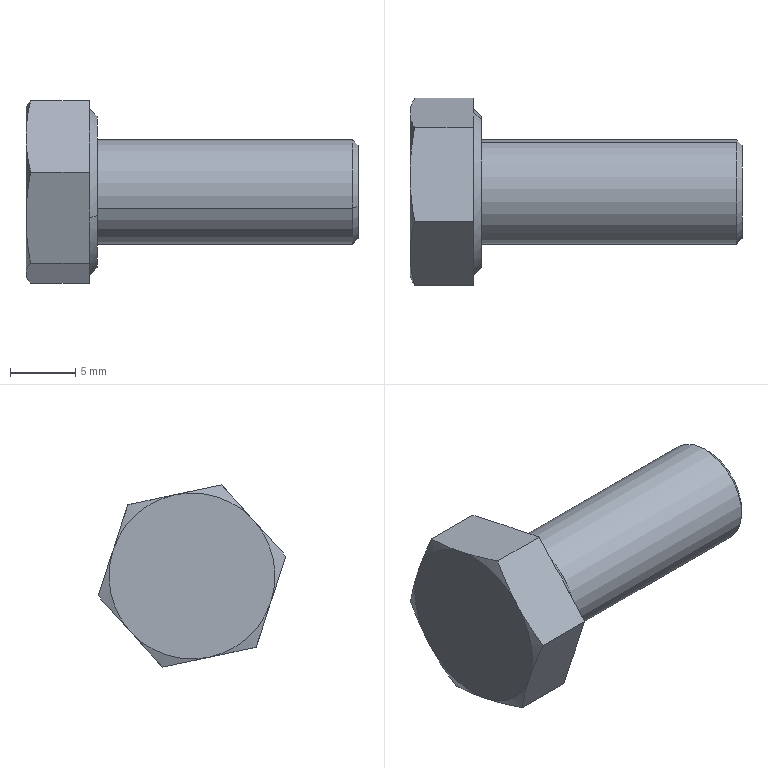Part | NX | features BREP 1 | 1 solid | 27 faces | box 25.45 x 14.378 x 13.98 mm | volume 1753 mm3 | plane 15 | cone 10 | cylinder 2 | commonest cylinder face diameters 8 x2
STEP:
#1=CARTESIAN_POINT('',(16.7,-2.901,82.764));
#2=VERTEX_POINT('',#1);
#3=CARTESIAN_POINT('',(16.7,3.946,84.989));
#4=VERTEX_POINT('',#3);
#5=CARTESIAN_POINT('',(16.7,0.5226,83.877));
#6=DIRECTION('',(1.,0.,0.));
#7=DIRECTION('',(0.,-0.9511,-0.309));
#8=AXIS2_PLACEMENT_3D('',#5,#6,#7);
#9=CIRCLE('',#8,3.6);
#10=EDGE_CURVE('',#2,#4,#9,.T.);
#11=ORIENTED_EDGE('',*,*,#10,.F.);
#12=CARTESIAN_POINT('',(16.3,-3.282,82.641));
#13=VERTEX_POINT('',#12);
#14=CARTESIAN_POINT('',(16.7,-2.901,82.764));
#15=DIRECTION('',(-0.7071,-0.6725,-0.2185));
#16=VECTOR('',#15,1000.);
#17=LINE('',#14,#16);
#18=EDGE_CURVE('',#2,#13,#17,.T.);
#19=ORIENTED_EDGE('',*,*,#18,.T.);
#20=CARTESIAN_POINT('',(16.3,4.327,85.113));
#21=VERTEX_POINT('',#20);
#22=CARTESIAN_POINT('',(16.3,0.5226,83.877));
#23=DIRECTION('',(-1.,0.,0.));
#24=DIRECTION('',(0.,-0.9511,-0.309));
#25=AXIS2_PLACEMENT_3D('',#22,#23,#24);
#26=CIRCLE('',#25,4.);
#27=EDGE_CURVE('',#21,#13,#26,.T.);
#28=ORIENTED_EDGE('',*,*,#27,.F.);
#29=CARTESIAN_POINT('',(16.7,3.946,84.989));
#30=DIRECTION('',(-0.7071,0.6725,0.2185));
#31=VECTOR('',#30,1000.);
#32=LINE('',#29,#31);
#33=EDGE_CURVE('',#4,#21,#32,.T.);
#34=ORIENTED_EDGE('',*,*,#33,.F.);
#35=EDGE_LOOP('',(#11,#19,#28,#34));
#36=FACE_BOUND('',#35,.T.);
#37=CARTESIAN_POINT('',(16.7,0.5226,83.877));
#38=DIRECTION('',(-1.,0.,0.));
#39=DIRECTION('',(0.,-0.9511,-0.309));
#40=AXIS2_PLACEMENT_3D('',#37,#38,#39);
#41=CONICAL_SURFACE('',#40,3.6,0.7854);
#42=ADVANCED_FACE('',(#36),#41,.T.);
#43=ORIENTED_EDGE('',*,*,#27,.T.);
#44=CARTESIAN_POINT('',(-3.3,-3.282,82.641));
#45=VERTEX_POINT('',#44);
#46=CARTESIAN_POINT('',(16.7,-3.282,82.641));
#47=DIRECTION('',(-1.,0.,0.));
#48=VECTOR('',#47,1000.);
#49=LINE('',#46,#48);
#50=EDGE_CURVE('',#13,#45,#49,.T.);
#51=ORIENTED_EDGE('',*,*,#50,.T.);
#52=CARTESIAN_POINT('',(-3.3,4.327,85.113));
#53=VERTEX_POINT('',#52);
#54=CARTESIAN_POINT('',(-3.3,0.5226,83.877));
#55=DIRECTION('',(1.,0.,0.));
#56=DIRECTION('',(0.,-0.9511,-0.309));
#57=AXIS2_PLACEMENT_3D('',#54,#55,#56);
#58=CIRCLE('',#57,4.);
#59=EDGE_CURVE('',#45,#53,#58,.T.);
#60=ORIENTED_EDGE('',*,*,#59,.T.);
#61=CARTESIAN_POINT('',(16.7,4.327,85.113));
#62=DIRECTION('',(-1.,0.,0.));
#63=VECTOR('',#62,1000.);
#64=LINE('',#61,#63);
#65=EDGE_CURVE('',#21,#53,#64,.T.);
#66=ORIENTED_EDGE('',*,*,#65,.F.);
#67=EDGE_LOOP('',(#43,#51,#60,#66));
#68=FACE_BOUND('',#67,.T.);
#69=CARTESIAN_POINT('',(16.7,0.5226,83.877));
#70=DIRECTION('',(-1.,0.,0.));
#71=DIRECTION('',(0.,-0.9511,-0.309));
#72=AXIS2_PLACEMENT_3D('',#69,#70,#71);
#73=CYLINDRICAL_SURFACE('',#72,4.);
#74=ADVANCED_FACE('',(#68),#73,.T.);
#75=CARTESIAN_POINT('',(-3.3,6.053,85.674));
#76=VERTEX_POINT('',#75);
#77=CARTESIAN_POINT('',(-3.3,-5.008,82.08));
#78=VERTEX_POINT('',#77);
#79=CARTESIAN_POINT('',(-3.3,0.5226,83.877));
#80=DIRECTION('',(-1.,0.,0.));
#81=DIRECTION('',(0.,0.9511,0.309));
#82=AXIS2_PLACEMENT_3D('',#79,#80,#81);
#83=CIRCLE('',#82,5.815);
#84=EDGE_CURVE('',#76,#78,#83,.T.);
#85=ORIENTED_EDGE('',*,*,#84,.T.);
#86=CARTESIAN_POINT('',(-3.85,-5.531,81.91));
#87=VERTEX_POINT('',#86);
#88=CARTESIAN_POINT('',(-3.9,-5.578,81.894));
#89=DIRECTION('',(-0.7071,-0.6725,-0.2185));
#90=VECTOR('',#89,1000.);
#91=LINE('',#88,#90);
#92=EDGE_CURVE('',#78,#87,#91,.T.);
#93=ORIENTED_EDGE('',*,*,#92,.T.);
#94=CARTESIAN_POINT('',(-3.9,-5.284,81.15));
#95=VERTEX_POINT('',#94);
#96=CARTESIAN_POINT('',(-3.85,-5.531,81.91));
#97=CARTESIAN_POINT('',(-3.85,-5.448,81.656));
#98=CARTESIAN_POINT('',(-3.867,-5.366,81.403));
#99=CARTESIAN_POINT('',(-3.9,-5.284,81.15));
#100=B_SPLINE_CURVE_WITH_KNOTS('',3,(#96,#97,#98,#99),.UNSPECIFIED.,.F.,.F.,(4,4),(0.,1.),.PIECEWISE_BEZIER_KNOTS.);
#101=EDGE_CURVE('',#87,#95,#100,.T.);
#102=ORIENTED_EDGE('',*,*,#101,.T.);
#103=CARTESIAN_POINT('',(-3.9,-1.583,77.817));
#104=VERTEX_POINT('',#103);
#105=CARTESIAN_POINT('',(-3.9,0.5226,83.877));
#106=DIRECTION('',(-1.,0.,0.));
#107=DIRECTION('',(0.,0.9511,0.309));
#108=AXIS2_PLACEMENT_3D('',#105,#106,#107);
#109=CIRCLE('',#108,6.415);
#110=EDGE_CURVE('',#104,#95,#109,.T.);
#111=ORIENTED_EDGE('',*,*,#110,.F.);
#112=CARTESIAN_POINT('',(-3.9,-0.01885,77.485));
#113=VERTEX_POINT('',#112);
#114=CARTESIAN_POINT('',(-3.9,-1.583,77.817));
#115=CARTESIAN_POINT('',(-3.834,-1.061,77.706));
#116=CARTESIAN_POINT('',(-3.834,-0.5401,77.595));
#117=CARTESIAN_POINT('',(-3.9,-0.01885,77.485));
#118=B_SPLINE_CURVE_WITH_KNOTS('',3,(#114,#115,#116,#117),.UNSPECIFIED.,.F.,.F.,(4,4),(0.,0.001599),.UNSPECIFIED.);
#119=EDGE_CURVE('',#104,#113,#118,.T.);
#120=ORIENTED_EDGE('',*,*,#119,.T.);
#121=CARTESIAN_POINT('',(-3.9,4.718,79.024));
#122=VERTEX_POINT('',#121);
#123=CARTESIAN_POINT('',(-3.9,0.5226,83.877));
#124=DIRECTION('',(-1.,0.,0.));
#125=DIRECTION('',(0.,0.9511,0.309));
#126=AXIS2_PLACEMENT_3D('',#123,#124,#125);
#127=CIRCLE('',#126,6.415);
#128=EDGE_CURVE('',#122,#113,#127,.T.);
#129=ORIENTED_EDGE('',*,*,#128,.F.);
#130=CARTESIAN_POINT('',(-3.9,5.788,80.212));
#131=VERTEX_POINT('',#130);
#132=CARTESIAN_POINT('',(-3.9,4.718,79.024));
#133=CARTESIAN_POINT('',(-3.834,5.074,79.42));
#134=CARTESIAN_POINT('',(-3.834,5.431,79.816));
#135=CARTESIAN_POINT('',(-3.9,5.788,80.212));
#136=B_SPLINE_CURVE_WITH_KNOTS('',3,(#132,#133,#134,#135),.UNSPECIFIED.,.F.,.F.,(4,4),(0.,0.001599),.UNSPECIFIED.);
#137=EDGE_CURVE('',#122,#131,#136,.T.);
#138=ORIENTED_EDGE('',*,*,#137,.T.);
#139=CARTESIAN_POINT('',(-3.9,6.823,85.083));
#140=VERTEX_POINT('',#139);
#141=CARTESIAN_POINT('',(-3.9,0.5226,83.877));
#142=DIRECTION('',(-1.,0.,0.));
#143=DIRECTION('',(0.,0.9511,0.309));
#144=AXIS2_PLACEMENT_3D('',#141,#142,#143);
#145=CIRCLE('',#144,6.415);
#146=EDGE_CURVE('',#140,#131,#145,.T.);
#147=ORIENTED_EDGE('',*,*,#146,.F.);
#148=CARTESIAN_POINT('',(-3.85,6.576,85.844));
#149=VERTEX_POINT('',#148);
#150=CARTESIAN_POINT('',(-3.9,6.823,85.083));
#151=CARTESIAN_POINT('',(-3.867,6.741,85.337));
#152=CARTESIAN_POINT('',(-3.85,6.658,85.59));
#153=CARTESIAN_POINT('',(-3.85,6.576,85.844));
#154=B_SPLINE_CURVE_WITH_KNOTS('',3,(#150,#151,#152,#153),.UNSPECIFIED.,.F.,.F.,(4,4),(0.,1.),.PIECEWISE_BEZIER_KNOTS.);
#155=EDGE_CURVE('',#140,#149,#154,.T.);
#156=ORIENTED_EDGE('',*,*,#155,.T.);
#157=CARTESIAN_POINT('',(-3.9,6.624,85.859));
#158=DIRECTION('',(-0.7071,0.6725,0.2185));
#159=VECTOR('',#158,1000.);
#160=LINE('',#157,#159);
#161=EDGE_CURVE('',#76,#149,#160,.T.);
#162=ORIENTED_EDGE('',*,*,#161,.F.);
#163=EDGE_LOOP('',(#85,#93,#102,#111,#120,#129,#138,#147,#156,#162));
#164=FACE_BOUND('',#163,.T.);
#165=CARTESIAN_POINT('',(-3.9,0.5226,83.877));
#166=DIRECTION('',(-1.,0.,0.));
#167=DIRECTION('',(0.,-0.9511,-0.309));
#168=AXIS2_PLACEMENT_3D('',#165,#166,#167);
#169=CONICAL_SURFACE('',#168,6.415,0.7854);
#170=ADVANCED_FACE('',(#164),#169,.T.);
#171=ORIENTED_EDGE('',*,*,#84,.F.);
#172=CARTESIAN_POINT('',(-3.3,0.5226,83.877));
#173=DIRECTION('',(-1.,0.,0.));
#174=DIRECTION('',(0.,0.9511,0.309));
#175=AXIS2_PLACEMENT_3D('',#172,#173,#174);
#176=CIRCLE('',#175,5.815);
#177=EDGE_CURVE('',#78,#76,#176,.T.);
#178=ORIENTED_EDGE('',*,*,#177,.F.);
#179=EDGE_LOOP('',(#171,#178));
#180=FACE_BOUND('',#179,.T.);
#181=CARTESIAN_POINT('',(-3.3,0.5226,83.877));
#182=DIRECTION('',(1.,0.,0.));
#183=DIRECTION('',(0.,-0.9511,-0.309));
#184=AXIS2_PLACEMENT_3D('',#181,#182,#183);
#185=CIRCLE('',#184,4.);
#186=EDGE_CURVE('',#53,#45,#185,.T.);
#187=ORIENTED_EDGE('',*,*,#186,.F.);
#188=ORIENTED_EDGE('',*,*,#59,.F.);
#189=EDGE_LOOP('',(#187,#188));
#190=FACE_BOUND('',#189,.T.);
#191=CARTESIAN_POINT('',(-3.3,-6.666,85.405));
#192=DIRECTION('',(1.,0.,0.));
#193=DIRECTION('',(0.,0.9511,0.309));
#194=AXIS2_PLACEMENT_3D('',#191,#192,#193);
#195=PLANE('',#194);
#196=ADVANCED_FACE('',(#180,#190),#195,.T.);
#197=CARTESIAN_POINT('',(-8.392,-6.666,85.405));
#198=VERTEX_POINT('',#197);
#199=CARTESIAN_POINT('',(-8.75,-4.208,88.136));
#200=VERTEX_POINT('',#199);
#201=CARTESIAN_POINT('',(-8.392,-6.666,85.405));
#202=CARTESIAN_POINT('',(-8.613,-5.853,86.308));
#203=CARTESIAN_POINT('',(-8.75,-5.035,87.217));
#204=CARTESIAN_POINT('',(-8.75,-4.208,88.136));
#205=B_SPLINE_CURVE_WITH_KNOTS('',3,(#201,#202,#203,#204),.UNSPECIFIED.,.F.,.F.,(4,4),(0.,0.003692),.UNSPECIFIED.);
#206=EDGE_CURVE('',#198,#200,#205,.T.);
#207=ORIENTED_EDGE('',*,*,#206,.F.);
#208=CARTESIAN_POINT('',(-3.9,-6.666,85.405));
#209=VERTEX_POINT('',#208);
#210=CARTESIAN_POINT('',(-3.3,-6.666,85.405));
#211=DIRECTION('',(-1.,0.,0.));
#212=VECTOR('',#211,1000.);
#213=LINE('',#210,#212);
#214=EDGE_CURVE('',#209,#198,#213,.T.);
#215=ORIENTED_EDGE('',*,*,#214,.F.);
#216=CARTESIAN_POINT('',(-3.9,-4.742,87.542));
#217=VERTEX_POINT('',#216);
#218=CARTESIAN_POINT('',(-3.9,-1.749,90.867));
#219=DIRECTION('',(0.,-0.6691,-0.7431));
#220=VECTOR('',#219,1000.);
#221=LINE('',#218,#220);
#222=EDGE_CURVE('',#217,#209,#221,.T.);
#223=ORIENTED_EDGE('',*,*,#222,.F.);
#224=CARTESIAN_POINT('',(-3.9,-3.673,88.73));
#225=VERTEX_POINT('',#224);
#226=CARTESIAN_POINT('',(-3.9,-3.673,88.73));
#227=CARTESIAN_POINT('',(-3.834,-4.029,88.334));
#228=CARTESIAN_POINT('',(-3.834,-4.386,87.938));
#229=CARTESIAN_POINT('',(-3.9,-4.742,87.542));
#230=B_SPLINE_CURVE_WITH_KNOTS('',3,(#226,#227,#228,#229),.UNSPECIFIED.,.F.,.F.,(4,4),(0.,0.001599),.UNSPECIFIED.);
#231=EDGE_CURVE('',#225,#217,#230,.T.);
#232=ORIENTED_EDGE('',*,*,#231,.F.);
#233=CARTESIAN_POINT('',(-3.9,-1.749,90.867));
#234=VERTEX_POINT('',#233);
#235=CARTESIAN_POINT('',(-3.9,-1.749,90.867));
#236=DIRECTION('',(0.,-0.6691,-0.7431));
#237=VECTOR('',#236,1000.);
#238=LINE('',#235,#237);
#239=EDGE_CURVE('',#234,#225,#238,.T.);
#240=ORIENTED_EDGE('',*,*,#239,.F.);
#241=CARTESIAN_POINT('',(-8.392,-1.749,90.867));
#242=VERTEX_POINT('',#241);
#243=CARTESIAN_POINT('',(-3.3,-1.749,90.867));
#244=DIRECTION('',(-1.,0.,0.));
#245=VECTOR('',#244,1000.);
#246=LINE('',#243,#245);
#247=EDGE_CURVE('',#234,#242,#246,.T.);
#248=ORIENTED_EDGE('',*,*,#247,.T.);
#249=CARTESIAN_POINT('',(-8.75,-4.208,88.136));
#250=CARTESIAN_POINT('',(-8.75,-3.38,89.055));
#251=CARTESIAN_POINT('',(-8.613,-2.562,89.964));
#252=CARTESIAN_POINT('',(-8.392,-1.749,90.867));
#253=B_SPLINE_CURVE_WITH_KNOTS('',3,(#249,#250,#251,#252),.UNSPECIFIED.,.F.,.F.,(4,4),(0.,0.003692),.UNSPECIFIED.);
#254=EDGE_CURVE('',#200,#242,#253,.T.);
#255=ORIENTED_EDGE('',*,*,#254,.F.);
#256=EDGE_LOOP('',(#207,#215,#223,#232,#240,#248,#255));
#257=FACE_BOUND('',#256,.T.);
#258=CARTESIAN_POINT('',(-3.3,-1.749,90.867));
#259=DIRECTION('',(0.,0.7431,-0.6691));
#260=DIRECTION('',(0.,-0.6691,-0.7431));
#261=AXIS2_PLACEMENT_3D('',#258,#259,#260);
#262=PLANE('',#261);
#263=ADVANCED_FACE('',(#257),#262,.F.);
#264=CARTESIAN_POINT('',(-8.392,-4.395,78.415));
#265=VERTEX_POINT('',#264);
#266=CARTESIAN_POINT('',(-8.75,-5.531,81.91));
#267=VERTEX_POINT('',#266);
#268=CARTESIAN_POINT('',(-8.392,-4.395,78.415));
#269=CARTESIAN_POINT('',(-8.613,-4.771,79.57));
#270=CARTESIAN_POINT('',(-8.75,-5.149,80.734));
#271=CARTESIAN_POINT('',(-8.75,-5.531,81.91));
#272=B_SPLINE_CURVE_WITH_KNOTS('',3,(#268,#269,#270,#271),.UNSPECIFIED.,.F.,.F.,(4,4),(0.,0.003692),.UNSPECIFIED.);
#273=EDGE_CURVE('',#265,#267,#272,.T.);
#274=ORIENTED_EDGE('',*,*,#273,.F.);
#275=CARTESIAN_POINT('',(-3.9,-4.395,78.415));
#276=VERTEX_POINT('',#275);
#277=CARTESIAN_POINT('',(-3.3,-4.395,78.415));
#278=DIRECTION('',(-1.,0.,0.));
#279=VECTOR('',#278,1000.);
#280=LINE('',#277,#279);
#281=EDGE_CURVE('',#276,#265,#280,.T.);
#282=ORIENTED_EDGE('',*,*,#281,.F.);
#283=CARTESIAN_POINT('',(-3.9,-6.666,85.405));
#284=DIRECTION('',(0.,0.309,-0.9511));
#285=VECTOR('',#284,1000.);
#286=LINE('',#283,#285);
#287=EDGE_CURVE('',#95,#276,#286,.T.);
#288=ORIENTED_EDGE('',*,*,#287,.F.);
#289=ORIENTED_EDGE('',*,*,#101,.F.);
#290=CARTESIAN_POINT('',(-3.9,-5.778,82.67));
#291=VERTEX_POINT('',#290);
#292=CARTESIAN_POINT('',(-3.9,-5.778,82.67));
#293=CARTESIAN_POINT('',(-3.867,-5.695,82.417));
#294=CARTESIAN_POINT('',(-3.85,-5.613,82.163));
#295=CARTESIAN_POINT('',(-3.85,-5.531,81.91));
#296=B_SPLINE_CURVE_WITH_KNOTS('',3,(#292,#293,#294,#295),.UNSPECIFIED.,.F.,.F.,(4,4),(0.,1.),.PIECEWISE_BEZIER_KNOTS.);
#297=EDGE_CURVE('',#291,#87,#296,.T.);
#298=ORIENTED_EDGE('',*,*,#297,.F.);
#299=CARTESIAN_POINT('',(-3.9,-6.666,85.405));
#300=DIRECTION('',(0.,0.309,-0.9511));
#301=VECTOR('',#300,1000.);
#302=LINE('',#299,#301);
#303=EDGE_CURVE('',#209,#291,#302,.T.);
#304=ORIENTED_EDGE('',*,*,#303,.F.);
#305=ORIENTED_EDGE('',*,*,#214,.T.);
#306=CARTESIAN_POINT('',(-8.75,-5.531,81.91));
#307=CARTESIAN_POINT('',(-8.75,-5.913,83.086));
#308=CARTESIAN_POINT('',(-8.613,-6.291,84.249));
#309=CARTESIAN_POINT('',(-8.392,-6.666,85.405));
#310=B_SPLINE_CURVE_WITH_KNOTS('',3,(#306,#307,#308,#309),.UNSPECIFIED.,.F.,.F.,(4,4),(0.,0.003692),.UNSPECIFIED.);
#311=EDGE_CURVE('',#267,#198,#310,.T.);
#312=ORIENTED_EDGE('',*,*,#311,.F.);
#313=EDGE_LOOP('',(#274,#282,#288,#289,#298,#304,#305,#312));
#314=FACE_BOUND('',#313,.T.);
#315=CARTESIAN_POINT('',(-3.3,-6.666,85.405));
#316=DIRECTION('',(0.,0.9511,0.309));
#317=DIRECTION('',(0.,0.309,-0.9511));
#318=AXIS2_PLACEMENT_3D('',#315,#316,#317);
#319=PLANE('',#318);
#320=ADVANCED_FACE('',(#314),#319,.F.);
#321=CARTESIAN_POINT('',(-8.392,2.794,76.887));
#322=VERTEX_POINT('',#321);
#323=CARTESIAN_POINT('',(-8.75,-0.8008,77.651));
#324=VERTEX_POINT('',#323);
#325=CARTESIAN_POINT('',(-8.392,2.794,76.887));
#326=CARTESIAN_POINT('',(-8.613,1.605,77.139));
#327=CARTESIAN_POINT('',(-8.75,0.4088,77.394));
#328=CARTESIAN_POINT('',(-8.75,-0.8008,77.651));
#329=B_SPLINE_CURVE_WITH_KNOTS('',3,(#325,#326,#327,#328),.UNSPECIFIED.,.F.,.F.,(4,4),(0.,0.003692),.UNSPECIFIED.);
#330=EDGE_CURVE('',#322,#324,#329,.T.);
#331=ORIENTED_EDGE('',*,*,#330,.F.);
#332=CARTESIAN_POINT('',(-3.9,2.794,76.887));
#333=VERTEX_POINT('',#332);
#334=CARTESIAN_POINT('',(-3.3,2.794,76.887));
#335=DIRECTION('',(-1.,0.,0.));
#336=VECTOR('',#335,1000.);
#337=LINE('',#334,#336);
#338=EDGE_CURVE('',#333,#322,#337,.T.);
#339=ORIENTED_EDGE('',*,*,#338,.F.);
#340=CARTESIAN_POINT('',(-3.9,-4.395,78.415));
#341=DIRECTION('',(0.,0.9781,-0.2079));
#342=VECTOR('',#341,1000.);
#343=LINE('',#340,#342);
#344=EDGE_CURVE('',#113,#333,#343,.T.);
#345=ORIENTED_EDGE('',*,*,#344,.F.);
#346=ORIENTED_EDGE('',*,*,#119,.F.);
#347=CARTESIAN_POINT('',(-3.9,-4.395,78.415));
#348=DIRECTION('',(0.,0.9781,-0.2079));
#349=VECTOR('',#348,1000.);
#350=LINE('',#347,#349);
#351=EDGE_CURVE('',#276,#104,#350,.T.);
#352=ORIENTED_EDGE('',*,*,#351,.F.);
#353=ORIENTED_EDGE('',*,*,#281,.T.);
#354=CARTESIAN_POINT('',(-8.75,-0.8008,77.651));
#355=CARTESIAN_POINT('',(-8.75,-2.01,77.908));
#356=CARTESIAN_POINT('',(-8.613,-3.207,78.162));
#357=CARTESIAN_POINT('',(-8.392,-4.395,78.415));
#358=B_SPLINE_CURVE_WITH_KNOTS('',3,(#354,#355,#356,#357),.UNSPECIFIED.,.F.,.F.,(4,4),(0.,0.003692),.UNSPECIFIED.);
#359=EDGE_CURVE('',#324,#265,#358,.T.);
#360=ORIENTED_EDGE('',*,*,#359,.F.);
#361=EDGE_LOOP('',(#331,#339,#345,#346,#352,#353,#360));
#362=FACE_BOUND('',#361,.T.);
#363=CARTESIAN_POINT('',(-3.3,-4.395,78.415));
#364=DIRECTION('',(0.,0.2079,0.9781));
#365=DIRECTION('',(0.,0.9781,-0.2079));
#366=AXIS2_PLACEMENT_3D('',#363,#364,#365);
#367=PLANE('',#366);
#368=ADVANCED_FACE('',(#362),#367,.F.);
#369=CARTESIAN_POINT('',(-8.392,7.712,82.349));
#370=VERTEX_POINT('',#369);
#371=CARTESIAN_POINT('',(-8.75,5.253,79.618));
#372=VERTEX_POINT('',#371);
#373=CARTESIAN_POINT('',(-8.392,7.712,82.349));
#374=CARTESIAN_POINT('',(-8.613,6.899,81.446));
#375=CARTESIAN_POINT('',(-8.75,6.08,80.537));
#376=CARTESIAN_POINT('',(-8.75,5.253,79.618));
#377=B_SPLINE_CURVE_WITH_KNOTS('',3,(#373,#374,#375,#376),.UNSPECIFIED.,.F.,.F.,(4,4),(0.,0.003692),.UNSPECIFIED.);
#378=EDGE_CURVE('',#370,#372,#377,.T.);
#379=ORIENTED_EDGE('',*,*,#378,.F.);
#380=CARTESIAN_POINT('',(-3.9,7.712,82.349));
#381=VERTEX_POINT('',#380);
#382=CARTESIAN_POINT('',(-3.3,7.712,82.349));
#383=DIRECTION('',(-1.,0.,0.));
#384=VECTOR('',#383,1000.);
#385=LINE('',#382,#384);
#386=EDGE_CURVE('',#381,#370,#385,.T.);
#387=ORIENTED_EDGE('',*,*,#386,.F.);
#388=CARTESIAN_POINT('',(-3.9,2.794,76.887));
#389=DIRECTION('',(0.,0.6691,0.7431));
#390=VECTOR('',#389,1000.);
#391=LINE('',#388,#390);
#392=EDGE_CURVE('',#131,#381,#391,.T.);
#393=ORIENTED_EDGE('',*,*,#392,.F.);
#394=ORIENTED_EDGE('',*,*,#137,.F.);
#395=CARTESIAN_POINT('',(-3.9,2.794,76.887));
#396=DIRECTION('',(0.,0.6691,0.7431));
#397=VECTOR('',#396,1000.);
#398=LINE('',#395,#397);
#399=EDGE_CURVE('',#333,#122,#398,.T.);
#400=ORIENTED_EDGE('',*,*,#399,.F.);
#401=ORIENTED_EDGE('',*,*,#338,.T.);
#402=CARTESIAN_POINT('',(-8.75,5.253,79.618));
#403=CARTESIAN_POINT('',(-8.75,4.425,78.699));
#404=CARTESIAN_POINT('',(-8.613,3.607,77.79));
#405=CARTESIAN_POINT('',(-8.392,2.794,76.887));
#406=B_SPLINE_CURVE_WITH_KNOTS('',3,(#402,#403,#404,#405),.UNSPECIFIED.,.F.,.F.,(4,4),(0.,0.003692),.UNSPECIFIED.);
#407=EDGE_CURVE('',#372,#322,#406,.T.);
#408=ORIENTED_EDGE('',*,*,#407,.F.);
#409=EDGE_LOOP('',(#379,#387,#393,#394,#400,#401,#408));
#410=FACE_BOUND('',#409,.T.);
#411=CARTESIAN_POINT('',(-3.3,2.794,76.887));
#412=DIRECTION('',(0.,-0.7431,0.6691));
#413=DIRECTION('',(0.,0.6691,0.7431));
#414=AXIS2_PLACEMENT_3D('',#411,#412,#413);
#415=PLANE('',#414);
#416=ADVANCED_FACE('',(#410),#415,.F.);
#417=CARTESIAN_POINT('',(-8.392,5.44,89.339));
#418=VERTEX_POINT('',#417);
#419=CARTESIAN_POINT('',(-8.75,6.576,85.844));
#420=VERTEX_POINT('',#419);
#421=CARTESIAN_POINT('',(-8.392,5.44,89.339));
#422=CARTESIAN_POINT('',(-8.613,5.816,88.183));
#423=CARTESIAN_POINT('',(-8.75,6.194,87.02));
#424=CARTESIAN_POINT('',(-8.75,6.576,85.844));
#425=B_SPLINE_CURVE_WITH_KNOTS('',3,(#421,#422,#423,#424),.UNSPECIFIED.,.F.,.F.,(4,4),(0.,0.003692),.UNSPECIFIED.);
#426=EDGE_CURVE('',#418,#420,#425,.T.);
#427=ORIENTED_EDGE('',*,*,#426,.F.);
#428=CARTESIAN_POINT('',(-3.9,5.44,89.339));
#429=VERTEX_POINT('',#428);
#430=CARTESIAN_POINT('',(-3.3,5.44,89.339));
#431=DIRECTION('',(-1.,0.,0.));
#432=VECTOR('',#431,1000.);
#433=LINE('',#430,#432);
#434=EDGE_CURVE('',#429,#418,#433,.T.);
#435=ORIENTED_EDGE('',*,*,#434,.F.);
#436=CARTESIAN_POINT('',(-3.9,6.329,86.604));
#437=VERTEX_POINT('',#436);
#438=CARTESIAN_POINT('',(-3.9,7.712,82.349));
#439=DIRECTION('',(0.,-0.309,0.9511));
#440=VECTOR('',#439,1000.);
#441=LINE('',#438,#440);
#442=EDGE_CURVE('',#437,#429,#441,.T.);
#443=ORIENTED_EDGE('',*,*,#442,.F.);
#444=CARTESIAN_POINT('',(-3.85,6.576,85.844));
#445=CARTESIAN_POINT('',(-3.85,6.494,86.097));
#446=CARTESIAN_POINT('',(-3.867,6.411,86.35));
#447=CARTESIAN_POINT('',(-3.9,6.329,86.604));
#448=B_SPLINE_CURVE_WITH_KNOTS('',3,(#444,#445,#446,#447),.UNSPECIFIED.,.F.,.F.,(4,4),(0.,1.),.PIECEWISE_BEZIER_KNOTS.);
#449=EDGE_CURVE('',#149,#437,#448,.T.);
#450=ORIENTED_EDGE('',*,*,#449,.F.);
#451=ORIENTED_EDGE('',*,*,#155,.F.);
#452=CARTESIAN_POINT('',(-3.9,7.712,82.349));
#453=DIRECTION('',(0.,-0.309,0.9511));
#454=VECTOR('',#453,1000.);
#455=LINE('',#452,#454);
#456=EDGE_CURVE('',#381,#140,#455,.T.);
#457=ORIENTED_EDGE('',*,*,#456,.F.);
#458=ORIENTED_EDGE('',*,*,#386,.T.);
#459=CARTESIAN_POINT('',(-8.75,6.576,85.844));
#460=CARTESIAN_POINT('',(-8.75,6.958,84.668));
#461=CARTESIAN_POINT('',(-8.613,7.336,83.504));
#462=CARTESIAN_POINT('',(-8.392,7.712,82.349));
#463=B_SPLINE_CURVE_WITH_KNOTS('',3,(#459,#460,#461,#462),.UNSPECIFIED.,.F.,.F.,(4,4),(0.,0.003692),.UNSPECIFIED.);
#464=EDGE_CURVE('',#420,#370,#463,.T.);
#465=ORIENTED_EDGE('',*,*,#464,.F.);
#466=EDGE_LOOP('',(#427,#435,#443,#450,#451,#457,#458,#465));
#467=FACE_BOUND('',#466,.T.);
#468=CARTESIAN_POINT('',(-3.3,7.712,82.349));
#469=DIRECTION('',(0.,-0.9511,-0.309));
#470=DIRECTION('',(1.,0.,0.));
#471=AXIS2_PLACEMENT_3D('',#468,#469,#470);
#472=PLANE('',#471);
#473=ADVANCED_FACE('',(#467),#472,.F.);
#474=CARTESIAN_POINT('',(-8.75,1.846,90.103));
#475=VERTEX_POINT('',#474);
#476=CARTESIAN_POINT('',(-8.392,-1.749,90.867));
#477=CARTESIAN_POINT('',(-8.613,-0.5601,90.614));
#478=CARTESIAN_POINT('',(-8.75,0.6364,90.36));
#479=CARTESIAN_POINT('',(-8.75,1.846,90.103));
#480=B_SPLINE_CURVE_WITH_KNOTS('',3,(#476,#477,#478,#479),.UNSPECIFIED.,.F.,.F.,(4,4),(0.,0.003692),.UNSPECIFIED.);
#481=EDGE_CURVE('',#242,#475,#480,.T.);
#482=ORIENTED_EDGE('',*,*,#481,.F.);
#483=ORIENTED_EDGE('',*,*,#247,.F.);
#484=CARTESIAN_POINT('',(-3.9,1.064,90.269));
#485=VERTEX_POINT('',#484);
#486=CARTESIAN_POINT('',(-3.9,5.44,89.339));
#487=DIRECTION('',(0.,-0.9781,0.2079));
#488=VECTOR('',#487,1000.);
#489=LINE('',#486,#488);
#490=EDGE_CURVE('',#485,#234,#489,.T.);
#491=ORIENTED_EDGE('',*,*,#490,.F.);
#492=CARTESIAN_POINT('',(-3.9,2.628,89.936));
#493=VERTEX_POINT('',#492);
#494=CARTESIAN_POINT('',(-3.9,2.628,89.936));
#495=CARTESIAN_POINT('',(-3.834,2.107,90.047));
#496=CARTESIAN_POINT('',(-3.834,1.585,90.158));
#497=CARTESIAN_POINT('',(-3.9,1.064,90.269));
#498=B_SPLINE_CURVE_WITH_KNOTS('',3,(#494,#495,#496,#497),.UNSPECIFIED.,.F.,.F.,(4,4),(0.,0.001599),.UNSPECIFIED.);
#499=EDGE_CURVE('',#493,#485,#498,.T.);
#500=ORIENTED_EDGE('',*,*,#499,.F.);
#501=CARTESIAN_POINT('',(-3.9,5.44,89.339));
#502=DIRECTION('',(0.,-0.9781,0.2079));
#503=VECTOR('',#502,1000.);
#504=LINE('',#501,#503);
#505=EDGE_CURVE('',#429,#493,#504,.T.);
#506=ORIENTED_EDGE('',*,*,#505,.F.);
#507=ORIENTED_EDGE('',*,*,#434,.T.);
#508=CARTESIAN_POINT('',(-8.75,1.846,90.103));
#509=CARTESIAN_POINT('',(-8.75,3.056,89.846));
#510=CARTESIAN_POINT('',(-8.613,4.252,89.591));
#511=CARTESIAN_POINT('',(-8.392,5.44,89.339));
#512=B_SPLINE_CURVE_WITH_KNOTS('',3,(#508,#509,#510,#511),.UNSPECIFIED.,.F.,.F.,(4,4),(0.,0.003692),.UNSPECIFIED.);
#513=EDGE_CURVE('',#475,#418,#512,.T.);
#514=ORIENTED_EDGE('',*,*,#513,.F.);
#515=EDGE_LOOP('',(#482,#483,#491,#500,#506,#507,#514));
#516=FACE_BOUND('',#515,.T.);
#517=CARTESIAN_POINT('',(-3.3,5.44,89.339));
#518=DIRECTION('',(0.,-0.2079,-0.9781));
#519=DIRECTION('',(0.,-0.9781,0.2079));
#520=AXIS2_PLACEMENT_3D('',#517,#518,#519);
#521=PLANE('',#520);
#522=ADVANCED_FACE('',(#516),#521,.F.);
#523=ORIENTED_EDGE('',*,*,#222,.T.);
#524=ORIENTED_EDGE('',*,*,#303,.T.);
#525=CARTESIAN_POINT('',(-3.9,0.5226,83.877));
#526=DIRECTION('',(-1.,0.,0.));
#527=DIRECTION('',(0.,0.9511,0.309));
#528=AXIS2_PLACEMENT_3D('',#525,#526,#527);
#529=CIRCLE('',#528,6.415);
#530=EDGE_CURVE('',#291,#217,#529,.T.);
#531=ORIENTED_EDGE('',*,*,#530,.T.);
#532=EDGE_LOOP('',(#523,#524,#531));
#533=FACE_BOUND('',#532,.T.);
#534=CARTESIAN_POINT('',(-3.9,2.505,77.776));
#535=DIRECTION('',(1.,0.,0.));
#536=DIRECTION('',(0.,0.9511,0.309));
#537=AXIS2_PLACEMENT_3D('',#534,#535,#536);
#538=PLANE('',#537);
#539=ADVANCED_FACE('',(#533),#538,.T.);
#540=ORIENTED_EDGE('',*,*,#287,.T.);
#541=ORIENTED_EDGE('',*,*,#351,.T.);
#542=ORIENTED_EDGE('',*,*,#110,.T.);
#543=EDGE_LOOP('',(#540,#541,#542));
#544=FACE_BOUND('',#543,.T.);
#545=CARTESIAN_POINT('',(-3.9,2.505,77.776));
#546=DIRECTION('',(1.,0.,0.));
#547=DIRECTION('',(0.,0.9511,0.309));
#548=AXIS2_PLACEMENT_3D('',#545,#546,#547);
#549=PLANE('',#548);
#550=ADVANCED_FACE('',(#544),#549,.T.);
#551=ORIENTED_EDGE('',*,*,#344,.T.);
#552=ORIENTED_EDGE('',*,*,#399,.T.);
#553=ORIENTED_EDGE('',*,*,#128,.T.);
#554=EDGE_LOOP('',(#551,#552,#553));
#555=FACE_BOUND('',#554,.T.);
#556=CARTESIAN_POINT('',(-3.9,2.505,77.776));
#557=DIRECTION('',(1.,0.,0.));
#558=DIRECTION('',(0.,0.9511,0.309));
#559=AXIS2_PLACEMENT_3D('',#556,#557,#558);
#560=PLANE('',#559);
#561=ADVANCED_FACE('',(#555),#560,.T.);
#562=ORIENTED_EDGE('',*,*,#392,.T.);
#563=ORIENTED_EDGE('',*,*,#456,.T.);
#564=ORIENTED_EDGE('',*,*,#146,.T.);
#565=EDGE_LOOP('',(#562,#563,#564));
#566=FACE_BOUND('',#565,.T.);
#567=CARTESIAN_POINT('',(-3.9,2.505,77.776));
#568=DIRECTION('',(1.,0.,0.));
#569=DIRECTION('',(0.,0.9511,0.309));
#570=AXIS2_PLACEMENT_3D('',#567,#568,#569);
#571=PLANE('',#570);
#572=ADVANCED_FACE('',(#566),#571,.T.);
#573=ORIENTED_EDGE('',*,*,#442,.T.);
#574=ORIENTED_EDGE('',*,*,#505,.T.);
#575=CARTESIAN_POINT('',(-3.9,0.5226,83.877));
#576=DIRECTION('',(-1.,0.,0.));
#577=DIRECTION('',(0.,0.9511,0.309));
#578=AXIS2_PLACEMENT_3D('',#575,#576,#577);
#579=CIRCLE('',#578,6.415);
#580=EDGE_CURVE('',#493,#437,#579,.T.);
#581=ORIENTED_EDGE('',*,*,#580,.T.);
#582=EDGE_LOOP('',(#573,#574,#581));
#583=FACE_BOUND('',#582,.T.);
#584=CARTESIAN_POINT('',(-3.9,2.505,77.776));
#585=DIRECTION('',(1.,0.,0.));
#586=DIRECTION('',(0.,0.9511,0.309));
#587=AXIS2_PLACEMENT_3D('',#584,#585,#586);
#588=PLANE('',#587);
#589=ADVANCED_FACE('',(#583),#588,.T.);
#590=ORIENTED_EDGE('',*,*,#239,.T.);
#591=CARTESIAN_POINT('',(-3.9,0.5226,83.877));
#592=DIRECTION('',(-1.,0.,0.));
#593=DIRECTION('',(0.,0.9511,0.309));
#594=AXIS2_PLACEMENT_3D('',#591,#592,#593);
#595=CIRCLE('',#594,6.415);
#596=EDGE_CURVE('',#225,#485,#595,.T.);
#597=ORIENTED_EDGE('',*,*,#596,.T.);
#598=ORIENTED_EDGE('',*,*,#490,.T.);
#599=EDGE_LOOP('',(#590,#597,#598));
#600=FACE_BOUND('',#599,.T.);
#601=CARTESIAN_POINT('',(-3.9,2.505,77.776));
#602=DIRECTION('',(1.,0.,0.));
#603=DIRECTION('',(0.,0.9511,0.309));
#604=AXIS2_PLACEMENT_3D('',#601,#602,#603);
#605=PLANE('',#604);
#606=ADVANCED_FACE('',(#600),#605,.T.);
#607=ORIENTED_EDGE('',*,*,#92,.F.);
#608=ORIENTED_EDGE('',*,*,#177,.T.);
#609=ORIENTED_EDGE('',*,*,#161,.T.);
#610=ORIENTED_EDGE('',*,*,#449,.T.);
#611=ORIENTED_EDGE('',*,*,#580,.F.);
#612=ORIENTED_EDGE('',*,*,#499,.T.);
#613=ORIENTED_EDGE('',*,*,#596,.F.);
#614=ORIENTED_EDGE('',*,*,#231,.T.);
#615=ORIENTED_EDGE('',*,*,#530,.F.);
#616=ORIENTED_EDGE('',*,*,#297,.T.);
#617=EDGE_LOOP('',(#607,#608,#609,#610,#611,#612,#613,#614,#615,#616));
#618=FACE_BOUND('',#617,.T.);
#619=CARTESIAN_POINT('',(-3.9,0.5226,83.877));
#620=DIRECTION('',(-1.,0.,0.));
#621=DIRECTION('',(0.,-0.9511,-0.309));
#622=AXIS2_PLACEMENT_3D('',#619,#620,#621);
#623=CONICAL_SURFACE('',#622,6.415,0.7854);
#624=ADVANCED_FACE('',(#618),#623,.T.);
#625=ORIENTED_EDGE('',*,*,#311,.T.);
#626=ORIENTED_EDGE('',*,*,#206,.T.);
#627=CARTESIAN_POINT('',(-8.75,0.5226,83.877));
#628=DIRECTION('',(1.,0.,0.));
#629=DIRECTION('',(0.,-0.9511,-0.309));
#630=AXIS2_PLACEMENT_3D('',#627,#628,#629);
#631=CIRCLE('',#630,6.365);
#632=EDGE_CURVE('',#200,#267,#631,.T.);
#633=ORIENTED_EDGE('',*,*,#632,.T.);
#634=EDGE_LOOP('',(#625,#626,#633));
#635=FACE_BOUND('',#634,.T.);
#636=CARTESIAN_POINT('',(-8.75,0.5226,83.877));
#637=DIRECTION('',(1.,0.,0.));
#638=DIRECTION('',(0.,0.9511,0.309));
#639=AXIS2_PLACEMENT_3D('',#636,#637,#638);
#640=CONICAL_SURFACE('',#639,6.365,1.222);
#641=ADVANCED_FACE('',(#635),#640,.T.);
#642=ORIENTED_EDGE('',*,*,#254,.T.);
#643=ORIENTED_EDGE('',*,*,#481,.T.);
#644=CARTESIAN_POINT('',(-8.75,0.5226,83.877));
#645=DIRECTION('',(1.,0.,0.));
#646=DIRECTION('',(0.,-0.9511,-0.309));
#647=AXIS2_PLACEMENT_3D('',#644,#645,#646);
#648=CIRCLE('',#647,6.365);
#649=EDGE_CURVE('',#475,#200,#648,.T.);
#650=ORIENTED_EDGE('',*,*,#649,.T.);
#651=EDGE_LOOP('',(#642,#643,#650));
#652=FACE_BOUND('',#651,.T.);
#653=CARTESIAN_POINT('',(-8.75,0.5226,83.877));
#654=DIRECTION('',(1.,0.,0.));
#655=DIRECTION('',(0.,0.9511,0.309));
#656=AXIS2_PLACEMENT_3D('',#653,#654,#655);
#657=CONICAL_SURFACE('',#656,6.365,1.222);
#658=ADVANCED_FACE('',(#652),#657,.T.);
#659=ORIENTED_EDGE('',*,*,#426,.T.);
#660=CARTESIAN_POINT('',(-8.75,0.5226,83.877));
#661=DIRECTION('',(1.,0.,0.));
#662=DIRECTION('',(0.,-0.9511,-0.309));
#663=AXIS2_PLACEMENT_3D('',#660,#661,#662);
#664=CIRCLE('',#663,6.365);
#665=EDGE_CURVE('',#420,#475,#664,.T.);
#666=ORIENTED_EDGE('',*,*,#665,.T.);
#667=ORIENTED_EDGE('',*,*,#513,.T.);
#668=EDGE_LOOP('',(#659,#666,#667));
#669=FACE_BOUND('',#668,.T.);
#670=CARTESIAN_POINT('',(-8.75,0.5226,83.877));
#671=DIRECTION('',(1.,0.,0.));
#672=DIRECTION('',(0.,0.9511,0.309));
#673=AXIS2_PLACEMENT_3D('',#670,#671,#672);
#674=CONICAL_SURFACE('',#673,6.365,1.222);
#675=ADVANCED_FACE('',(#669),#674,.T.);
#676=ORIENTED_EDGE('',*,*,#378,.T.);
#677=CARTESIAN_POINT('',(-8.75,0.5226,83.877));
#678=DIRECTION('',(-1.,0.,0.));
#679=DIRECTION('',(0.,0.9511,0.309));
#680=AXIS2_PLACEMENT_3D('',#677,#678,#679);
#681=CIRCLE('',#680,6.365);
#682=EDGE_CURVE('',#420,#372,#681,.T.);
#683=ORIENTED_EDGE('',*,*,#682,.F.);
#684=ORIENTED_EDGE('',*,*,#464,.T.);
#685=EDGE_LOOP('',(#676,#683,#684));
#686=FACE_BOUND('',#685,.T.);
#687=CARTESIAN_POINT('',(-8.75,0.5226,83.877));
#688=DIRECTION('',(1.,0.,0.));
#689=DIRECTION('',(0.,0.9511,0.309));
#690=AXIS2_PLACEMENT_3D('',#687,#688,#689);
#691=CONICAL_SURFACE('',#690,6.365,1.222);
#692=ADVANCED_FACE('',(#686),#691,.T.);
#693=ORIENTED_EDGE('',*,*,#330,.T.);
#694=CARTESIAN_POINT('',(-8.75,0.5226,83.877));
#695=DIRECTION('',(1.,0.,0.));
#696=DIRECTION('',(0.,-0.9511,-0.309));
#697=AXIS2_PLACEMENT_3D('',#694,#695,#696);
#698=CIRCLE('',#697,6.365);
#699=EDGE_CURVE('',#324,#372,#698,.T.);
#700=ORIENTED_EDGE('',*,*,#699,.T.);
#701=ORIENTED_EDGE('',*,*,#407,.T.);
#702=EDGE_LOOP('',(#693,#700,#701));
#703=FACE_BOUND('',#702,.T.);
#704=CARTESIAN_POINT('',(-8.75,0.5226,83.877));
#705=DIRECTION('',(1.,0.,0.));
#706=DIRECTION('',(0.,0.9511,0.309));
#707=AXIS2_PLACEMENT_3D('',#704,#705,#706);
#708=CONICAL_SURFACE('',#707,6.365,1.222);
#709=ADVANCED_FACE('',(#703),#708,.T.);
#710=ORIENTED_EDGE('',*,*,#359,.T.);
#711=ORIENTED_EDGE('',*,*,#273,.T.);
#712=CARTESIAN_POINT('',(-8.75,0.5226,83.877));
#713=DIRECTION('',(1.,0.,0.));
#714=DIRECTION('',(0.,-0.9511,-0.309));
#715=AXIS2_PLACEMENT_3D('',#712,#713,#714);
#716=CIRCLE('',#715,6.365);
#717=EDGE_CURVE('',#267,#324,#716,.T.);
#718=ORIENTED_EDGE('',*,*,#717,.T.);
#719=EDGE_LOOP('',(#710,#711,#718));
#720=FACE_BOUND('',#719,.T.);
#721=CARTESIAN_POINT('',(-8.75,0.5226,83.877));
#722=DIRECTION('',(1.,0.,0.));
#723=DIRECTION('',(0.,0.9511,0.309));
#724=AXIS2_PLACEMENT_3D('',#721,#722,#723);
#725=CONICAL_SURFACE('',#724,6.365,1.222);
#726=ADVANCED_FACE('',(#720),#725,.T.);
#727=ORIENTED_EDGE('',*,*,#717,.F.);
#728=ORIENTED_EDGE('',*,*,#632,.F.);
#729=ORIENTED_EDGE('',*,*,#649,.F.);
#730=ORIENTED_EDGE('',*,*,#665,.F.);
#731=ORIENTED_EDGE('',*,*,#682,.T.);
#732=ORIENTED_EDGE('',*,*,#699,.F.);
#733=EDGE_LOOP('',(#727,#728,#729,#730,#731,#732));
#734=FACE_BOUND('',#733,.T.);
#735=CARTESIAN_POINT('',(-8.75,-6.666,85.405));
#736=DIRECTION('',(1.,0.,0.));
#737=DIRECTION('',(0.,0.9511,0.309));
#738=AXIS2_PLACEMENT_3D('',#735,#736,#737);
#739=PLANE('',#738);
#740=ADVANCED_FACE('',(#734),#739,.F.);
#741=ORIENTED_EDGE('',*,*,#50,.F.);
#742=CARTESIAN_POINT('',(16.3,0.5226,83.877));
#743=DIRECTION('',(-1.,0.,0.));
#744=DIRECTION('',(0.,-0.9511,-0.309));
#745=AXIS2_PLACEMENT_3D('',#742,#743,#744);
#746=CIRCLE('',#745,4.);
#747=EDGE_CURVE('',#13,#21,#746,.T.);
#748=ORIENTED_EDGE('',*,*,#747,.T.);
#749=ORIENTED_EDGE('',*,*,#65,.T.);
#750=ORIENTED_EDGE('',*,*,#186,.T.);
#751=EDGE_LOOP('',(#741,#748,#749,#750));
#752=FACE_BOUND('',#751,.T.);
#753=CARTESIAN_POINT('',(16.7,0.5226,83.877));
#754=DIRECTION('',(-1.,0.,0.));
#755=DIRECTION('',(0.,-0.9511,-0.309));
#756=AXIS2_PLACEMENT_3D('',#753,#754,#755);
#757=CYLINDRICAL_SURFACE('',#756,4.);
#758=ADVANCED_FACE('',(#752),#757,.T.);
#759=CARTESIAN_POINT('',(16.7,0.5226,83.877));
#760=DIRECTION('',(1.,0.,0.));
#761=DIRECTION('',(0.,-0.9511,-0.309));
#762=AXIS2_PLACEMENT_3D('',#759,#760,#761);
#763=CIRCLE('',#762,3.6);
#764=EDGE_CURVE('',#4,#2,#763,.T.);
#765=ORIENTED_EDGE('',*,*,#764,.T.);
#766=ORIENTED_EDGE('',*,*,#10,.T.);
#767=EDGE_LOOP('',(#765,#766));
#768=FACE_BOUND('',#767,.T.);
#769=CARTESIAN_POINT('',(16.7,0.5226,83.877));
#770=DIRECTION('',(1.,0.,0.));
#771=DIRECTION('',(0.,0.9511,0.309));
#772=AXIS2_PLACEMENT_3D('',#769,#770,#771);
#773=PLANE('',#772);
#774=ADVANCED_FACE('',(#768),#773,.T.);
#775=ORIENTED_EDGE('',*,*,#18,.F.);
#776=ORIENTED_EDGE('',*,*,#764,.F.);
#777=ORIENTED_EDGE('',*,*,#33,.T.);
#778=ORIENTED_EDGE('',*,*,#747,.F.);
#779=EDGE_LOOP('',(#775,#776,#777,#778));
#780=FACE_BOUND('',#779,.T.);
#781=CARTESIAN_POINT('',(16.7,0.5226,83.877));
#782=DIRECTION('',(-1.,0.,0.));
#783=DIRECTION('',(0.,-0.9511,-0.309));
#784=AXIS2_PLACEMENT_3D('',#781,#782,#783);
#785=CONICAL_SURFACE('',#784,3.6,0.7854);
#786=ADVANCED_FACE('',(#780),#785,.T.);
#787=CLOSED_SHELL('',(#42,#74,#170,#196,#263,#320,#368,#416,#473,#522,#539,#550,#561,#572,#589,#606,#624,#641,#658,#675,#692,#709,#726,#740,#758,#774,#786));
#788=MANIFOLD_SOLID_BREP('',#787);
#789=(LENGTH_UNIT()NAMED_UNIT(*)SI_UNIT(.MILLI.,.METRE.));
#790=UNCERTAINTY_MEASURE_WITH_UNIT(LENGTH_MEASURE(0.0508),#789,'','');
#791=(NAMED_UNIT(*)PLANE_ANGLE_UNIT()SI_UNIT($,.RADIAN.));
#792=(NAMED_UNIT(*)SI_UNIT($,.STERADIAN.)SOLID_ANGLE_UNIT());
#793=(GEOMETRIC_REPRESENTATION_CONTEXT(3)GLOBAL_UNCERTAINTY_ASSIGNED_CONTEXT((#790))GLOBAL_UNIT_ASSIGNED_CONTEXT((#789,#791,#792))REPRESENTATION_CONTEXT('',''));
#794=ADVANCED_BREP_SHAPE_REPRESENTATION('',(#788),#793);